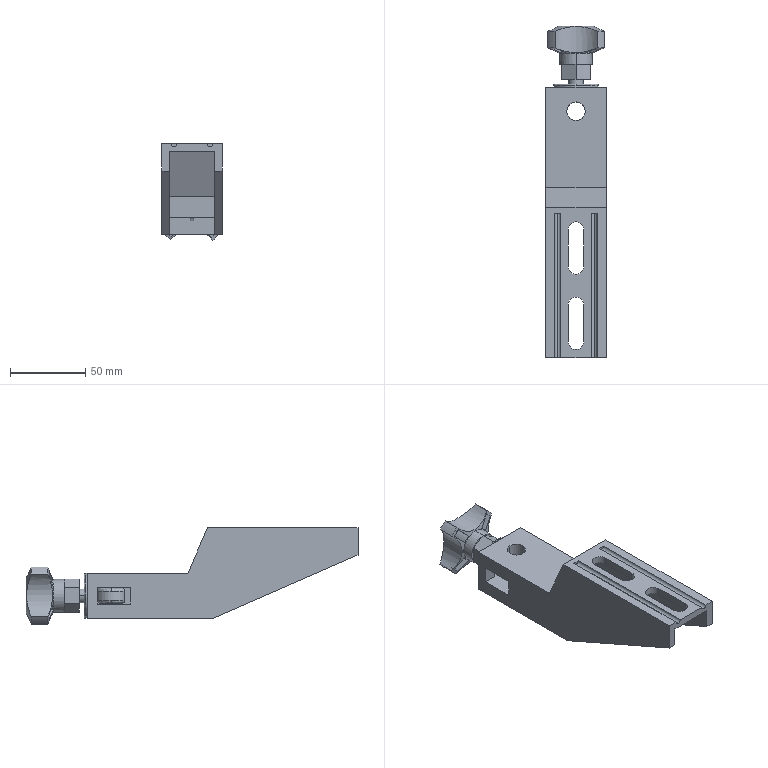Part | SolidWorks | 4 solids | 140 faces | box 40 x 220.567 x 63.886 mm | volume 127042 mm3 | plane 74 | cylinder 48 | spline 12 | cone 6 | commonest cylinder face diameters 4 x8 10.5 x6 12.2 x6 36 x5 23 x4 43 x4